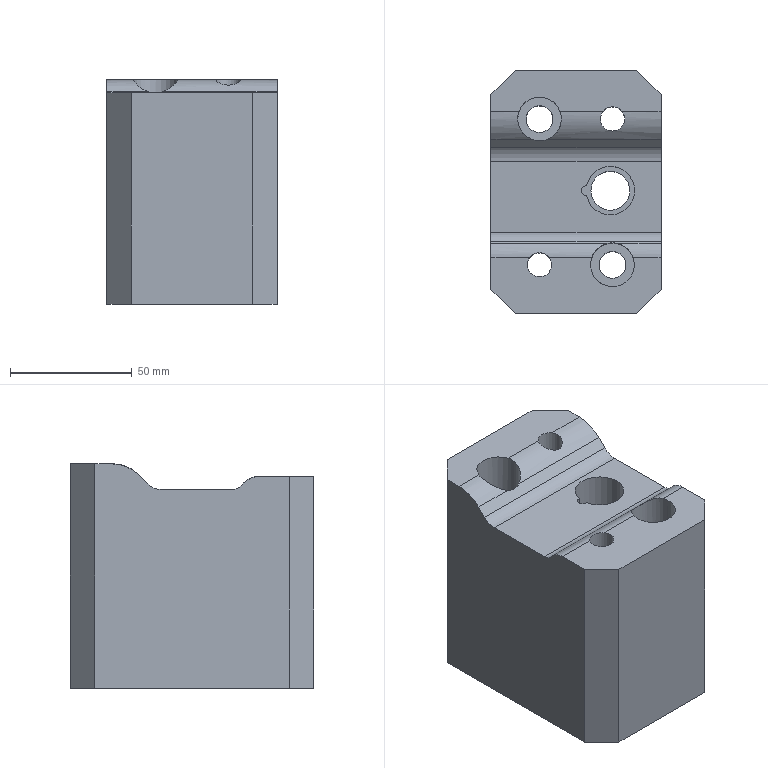Part | NX | features solid 2 | 1 solid | 34 faces | box 70 x 100 x 92.308 mm | volume 508143 mm3 | plane 18 | cylinder 16 | commonest cylinder face diameters 16 x4 10 x3 11 x2 18 x2 32 x2 4 x1
STEP:
#1=CARTESIAN_POINT('',(279.343,-472.51,86.708));
#2=VERTEX_POINT('',#1);
#3=CARTESIAN_POINT('',(279.343,-476.49,86.708));
#4=VERTEX_POINT('',#3);
#5=CARTESIAN_POINT('',(279.143,-474.5,86.708));
#6=DIRECTION('',(0.,0.,1.));
#7=DIRECTION('',(1.,0.,0.));
#8=AXIS2_PLACEMENT_3D('',#5,#6,#7);
#9=CIRCLE('',#8,2.);
#10=EDGE_CURVE('',#2,#4,#9,.T.);
#11=ORIENTED_EDGE('',*,*,#10,.F.);
#12=CARTESIAN_POINT('',(289.143,-474.5,86.708));
#13=DIRECTION('',(0.,0.,1.));
#14=DIRECTION('',(1.,0.,0.));
#15=AXIS2_PLACEMENT_3D('',#12,#13,#14);
#16=CIRCLE('',#15,10.);
#17=EDGE_CURVE('',#2,#4,#16,.F.);
#18=ORIENTED_EDGE('',*,*,#17,.T.);
#19=EDGE_LOOP('',(#11,#18));
#20=FACE_BOUND('',#19,.T.);
#21=CARTESIAN_POINT('',(240.,-491.596,86.708));
#22=VERTEX_POINT('',#21);
#23=CARTESIAN_POINT('',(240.,-462.454,86.708));
#24=VERTEX_POINT('',#23);
#25=CARTESIAN_POINT('',(240.,-475.,86.708));
#26=DIRECTION('',(0.,1.,0.));
#27=VECTOR('',#26,1000.);
#28=LINE('',#25,#27);
#29=EDGE_CURVE('',#22,#24,#28,.T.);
#30=ORIENTED_EDGE('',*,*,#29,.F.);
#31=CARTESIAN_POINT('',(310.,-491.596,86.708));
#32=VERTEX_POINT('',#31);
#33=CARTESIAN_POINT('',(240.,-491.596,86.708));
#34=CARTESIAN_POINT('',(263.333,-491.596,86.708));
#35=CARTESIAN_POINT('',(286.667,-491.596,86.708));
#36=CARTESIAN_POINT('',(310.,-491.596,86.708));
#37=B_SPLINE_CURVE_WITH_KNOTS('',3,(#33,#34,#35,#36),.UNSPECIFIED.,.F.,.F.,(4,4),(0.7902,0.8748),.UNSPECIFIED.);
#38=EDGE_CURVE('',#22,#32,#37,.T.);
#39=ORIENTED_EDGE('',*,*,#38,.T.);
#40=CARTESIAN_POINT('',(310.,-462.454,86.708));
#41=VERTEX_POINT('',#40);
#42=CARTESIAN_POINT('',(310.,-475.,86.708));
#43=DIRECTION('',(0.,-1.,0.));
#44=VECTOR('',#43,1000.);
#45=LINE('',#42,#44);
#46=EDGE_CURVE('',#41,#32,#45,.T.);
#47=ORIENTED_EDGE('',*,*,#46,.F.);
#48=CARTESIAN_POINT('',(310.,-462.454,86.708));
#49=CARTESIAN_POINT('',(286.667,-462.454,86.708));
#50=CARTESIAN_POINT('',(263.333,-462.454,86.708));
#51=CARTESIAN_POINT('',(240.,-462.454,86.708));
#52=B_SPLINE_CURVE_WITH_KNOTS('',3,(#48,#49,#50,#51),.UNSPECIFIED.,.F.,.F.,(4,4),(0.1252,0.2098),.UNSPECIFIED.);
#53=EDGE_CURVE('',#41,#24,#52,.T.);
#54=ORIENTED_EDGE('',*,*,#53,.T.);
#55=EDGE_LOOP('',(#30,#39,#47,#54));
#56=FACE_BOUND('',#55,.T.);
#57=CARTESIAN_POINT('',(426.488,227.578,86.708));
#58=DIRECTION('',(0.,0.,1.));
#59=DIRECTION('',(0.,-1.,0.));
#60=AXIS2_PLACEMENT_3D('',#57,#58,#59);
#61=PLANE('',#60);
#62=ADVANCED_FACE('',(#20,#56),#61,.T.);
#63=CARTESIAN_POINT('',(300.,-525.,5.));
#64=VERTEX_POINT('',#63);
#65=CARTESIAN_POINT('',(300.,-525.,92.008));
#66=VERTEX_POINT('',#65);
#67=CARTESIAN_POINT('',(300.,-525.,10.));
#68=DIRECTION('',(0.,0.,1.));
#69=VECTOR('',#68,1000.);
#70=LINE('',#67,#69);
#71=EDGE_CURVE('',#64,#66,#70,.T.);
#72=ORIENTED_EDGE('',*,*,#71,.T.);
#73=CARTESIAN_POINT('',(250.,-525.,92.008));
#74=VERTEX_POINT('',#73);
#75=CARTESIAN_POINT('',(250.,-525.,92.008));
#76=DIRECTION('',(-1.,0.,0.));
#77=VECTOR('',#76,1000.);
#78=LINE('',#75,#77);
#79=EDGE_CURVE('',#66,#74,#78,.T.);
#80=ORIENTED_EDGE('',*,*,#79,.T.);
#81=CARTESIAN_POINT('',(250.,-525.,5.));
#82=VERTEX_POINT('',#81);
#83=CARTESIAN_POINT('',(250.,-525.,10.));
#84=DIRECTION('',(0.,0.,-1.));
#85=VECTOR('',#84,1000.);
#86=LINE('',#83,#85);
#87=EDGE_CURVE('',#74,#82,#86,.T.);
#88=ORIENTED_EDGE('',*,*,#87,.T.);
#89=CARTESIAN_POINT('',(250.,-525.,5.));
#90=DIRECTION('',(1.,0.,0.));
#91=VECTOR('',#90,1000.);
#92=LINE('',#89,#91);
#93=EDGE_CURVE('',#82,#64,#92,.T.);
#94=ORIENTED_EDGE('',*,*,#93,.T.);
#95=EDGE_LOOP('',(#72,#80,#88,#94));
#96=FACE_BOUND('',#95,.T.);
#97=CARTESIAN_POINT('',(250.,-525.,10.));
#98=DIRECTION('',(0.,-1.,0.));
#99=DIRECTION('',(0.,0.,-1.));
#100=AXIS2_PLACEMENT_3D('',#97,#98,#99);
#101=PLANE('',#100);
#102=ADVANCED_FACE('',(#96),#101,.T.);
#103=CARTESIAN_POINT('',(240.,-515.,5.));
#104=VERTEX_POINT('',#103);
#105=CARTESIAN_POINT('',(240.,-515.,92.008));
#106=VERTEX_POINT('',#105);
#107=CARTESIAN_POINT('',(240.,-515.,10.));
#108=DIRECTION('',(0.,0.,1.));
#109=VECTOR('',#108,1000.);
#110=LINE('',#107,#109);
#111=EDGE_CURVE('',#104,#106,#110,.T.);
#112=ORIENTED_EDGE('',*,*,#111,.T.);
#113=CARTESIAN_POINT('',(240.,-502.176,92.008));
#114=VERTEX_POINT('',#113);
#115=CARTESIAN_POINT('',(240.,-475.,92.008));
#116=DIRECTION('',(0.,1.,0.));
#117=VECTOR('',#116,1000.);
#118=LINE('',#115,#117);
#119=EDGE_CURVE('',#106,#114,#118,.T.);
#120=ORIENTED_EDGE('',*,*,#119,.T.);
#121=CARTESIAN_POINT('',(240.,-496.288,89.423));
#122=VERTEX_POINT('',#121);
#123=CARTESIAN_POINT('',(240.,-502.176,84.008));
#124=DIRECTION('',(-1.,0.,0.));
#125=DIRECTION('',(0.,0.,1.));
#126=AXIS2_PLACEMENT_3D('',#123,#124,#125);
#127=CIRCLE('',#126,8.);
#128=EDGE_CURVE('',#114,#122,#127,.T.);
#129=ORIENTED_EDGE('',*,*,#128,.T.);
#130=CARTESIAN_POINT('',(240.,-495.276,88.323));
#131=VERTEX_POINT('',#130);
#132=CARTESIAN_POINT('',(240.,-446.959,35.79));
#133=DIRECTION('',(0.,0.677,-0.736));
#134=VECTOR('',#133,1000.);
#135=LINE('',#132,#134);
#136=EDGE_CURVE('',#122,#131,#135,.T.);
#137=ORIENTED_EDGE('',*,*,#136,.T.);
#138=CARTESIAN_POINT('',(240.,-491.596,91.708));
#139=DIRECTION('',(-1.,0.,0.));
#140=DIRECTION('',(0.,0.,1.));
#141=AXIS2_PLACEMENT_3D('',#138,#139,#140);
#142=CIRCLE('',#141,5.);
#143=EDGE_CURVE('',#22,#131,#142,.T.);
#144=ORIENTED_EDGE('',*,*,#143,.F.);
#145=ORIENTED_EDGE('',*,*,#29,.T.);
#146=CARTESIAN_POINT('',(240.,-456.76,89.089));
#147=VERTEX_POINT('',#146);
#148=CARTESIAN_POINT('',(240.,-462.454,94.708));
#149=DIRECTION('',(-1.,0.,0.));
#150=DIRECTION('',(0.,0.,1.));
#151=AXIS2_PLACEMENT_3D('',#148,#149,#150);
#152=CIRCLE('',#151,8.);
#153=EDGE_CURVE('',#147,#24,#152,.T.);
#154=ORIENTED_EDGE('',*,*,#153,.F.);
#155=CARTESIAN_POINT('',(240.,-453.348,92.546));
#156=VERTEX_POINT('',#155);
#157=CARTESIAN_POINT('',(240.,-505.299,39.898));
#158=DIRECTION('',(0.,0.7024,0.7118));
#159=VECTOR('',#158,1000.);
#160=LINE('',#157,#159);
#161=EDGE_CURVE('',#147,#156,#160,.T.);
#162=ORIENTED_EDGE('',*,*,#161,.T.);
#163=CARTESIAN_POINT('',(240.,-441.959,97.308));
#164=VERTEX_POINT('',#163);
#165=CARTESIAN_POINT('',(240.,-441.959,81.308));
#166=DIRECTION('',(-1.,0.,0.));
#167=DIRECTION('',(0.,0.,1.));
#168=AXIS2_PLACEMENT_3D('',#165,#166,#167);
#169=CIRCLE('',#168,16.);
#170=EDGE_CURVE('',#156,#164,#169,.T.);
#171=ORIENTED_EDGE('',*,*,#170,.T.);
#172=CARTESIAN_POINT('',(240.,-435.,97.308));
#173=VERTEX_POINT('',#172);
#174=CARTESIAN_POINT('',(240.,-475.,97.308));
#175=DIRECTION('',(0.,1.,0.));
#176=VECTOR('',#175,1000.);
#177=LINE('',#174,#176);
#178=EDGE_CURVE('',#164,#173,#177,.T.);
#179=ORIENTED_EDGE('',*,*,#178,.T.);
#180=CARTESIAN_POINT('',(240.,-435.,5.));
#181=VERTEX_POINT('',#180);
#182=CARTESIAN_POINT('',(240.,-435.,10.));
#183=DIRECTION('',(0.,0.,-1.));
#184=VECTOR('',#183,1000.);
#185=LINE('',#182,#184);
#186=EDGE_CURVE('',#173,#181,#185,.T.);
#187=ORIENTED_EDGE('',*,*,#186,.T.);
#188=CARTESIAN_POINT('',(240.,-475.,5.));
#189=DIRECTION('',(0.,-1.,0.));
#190=VECTOR('',#189,1000.);
#191=LINE('',#188,#190);
#192=EDGE_CURVE('',#181,#104,#191,.T.);
#193=ORIENTED_EDGE('',*,*,#192,.T.);
#194=EDGE_LOOP('',(#112,#120,#129,#137,#144,#145,#154,#162,#171,#179,#187,#193));
#195=FACE_BOUND('',#194,.T.);
#196=CARTESIAN_POINT('',(240.,-475.,10.));
#197=DIRECTION('',(-1.,0.,0.));
#198=DIRECTION('',(0.,0.,1.));
#199=AXIS2_PLACEMENT_3D('',#196,#197,#198);
#200=PLANE('',#199);
#201=ADVANCED_FACE('',(#195),#200,.T.);
#202=CARTESIAN_POINT('',(250.,-425.,5.));
#203=VERTEX_POINT('',#202);
#204=CARTESIAN_POINT('',(250.,-425.,97.308));
#205=VERTEX_POINT('',#204);
#206=CARTESIAN_POINT('',(250.,-425.,10.));
#207=DIRECTION('',(0.,0.,1.));
#208=VECTOR('',#207,1000.);
#209=LINE('',#206,#208);
#210=EDGE_CURVE('',#203,#205,#209,.T.);
#211=ORIENTED_EDGE('',*,*,#210,.T.);
#212=CARTESIAN_POINT('',(300.,-425.,97.308));
#213=VERTEX_POINT('',#212);
#214=CARTESIAN_POINT('',(250.,-425.,97.308));
#215=DIRECTION('',(1.,0.,0.));
#216=VECTOR('',#215,1000.);
#217=LINE('',#214,#216);
#218=EDGE_CURVE('',#205,#213,#217,.T.);
#219=ORIENTED_EDGE('',*,*,#218,.T.);
#220=CARTESIAN_POINT('',(300.,-425.,5.));
#221=VERTEX_POINT('',#220);
#222=CARTESIAN_POINT('',(300.,-425.,10.));
#223=DIRECTION('',(0.,0.,-1.));
#224=VECTOR('',#223,1000.);
#225=LINE('',#222,#224);
#226=EDGE_CURVE('',#213,#221,#225,.T.);
#227=ORIENTED_EDGE('',*,*,#226,.T.);
#228=CARTESIAN_POINT('',(250.,-425.,5.));
#229=DIRECTION('',(-1.,0.,0.));
#230=VECTOR('',#229,1000.);
#231=LINE('',#228,#230);
#232=EDGE_CURVE('',#221,#203,#231,.T.);
#233=ORIENTED_EDGE('',*,*,#232,.T.);
#234=EDGE_LOOP('',(#211,#219,#227,#233));
#235=FACE_BOUND('',#234,.T.);
#236=CARTESIAN_POINT('',(250.,-425.,10.));
#237=DIRECTION('',(0.,1.,0.));
#238=DIRECTION('',(0.,0.,1.));
#239=AXIS2_PLACEMENT_3D('',#236,#237,#238);
#240=PLANE('',#239);
#241=ADVANCED_FACE('',(#235),#240,.T.);
#242=CARTESIAN_POINT('',(310.,-496.288,89.423));
#243=VERTEX_POINT('',#242);
#244=CARTESIAN_POINT('',(310.,-502.176,92.008));
#245=VERTEX_POINT('',#244);
#246=CARTESIAN_POINT('',(310.,-502.176,84.008));
#247=DIRECTION('',(1.,0.,0.));
#248=DIRECTION('',(0.,0.,-1.));
#249=AXIS2_PLACEMENT_3D('',#246,#247,#248);
#250=CIRCLE('',#249,8.);
#251=EDGE_CURVE('',#243,#245,#250,.T.);
#252=ORIENTED_EDGE('',*,*,#251,.T.);
#253=CARTESIAN_POINT('',(310.,-515.,92.008));
#254=VERTEX_POINT('',#253);
#255=CARTESIAN_POINT('',(310.,-475.,92.008));
#256=DIRECTION('',(0.,-1.,0.));
#257=VECTOR('',#256,1000.);
#258=LINE('',#255,#257);
#259=EDGE_CURVE('',#245,#254,#258,.T.);
#260=ORIENTED_EDGE('',*,*,#259,.T.);
#261=CARTESIAN_POINT('',(310.,-515.,5.));
#262=VERTEX_POINT('',#261);
#263=CARTESIAN_POINT('',(310.,-515.,10.));
#264=DIRECTION('',(0.,0.,-1.));
#265=VECTOR('',#264,1000.);
#266=LINE('',#263,#265);
#267=EDGE_CURVE('',#254,#262,#266,.T.);
#268=ORIENTED_EDGE('',*,*,#267,.T.);
#269=CARTESIAN_POINT('',(310.,-435.,5.));
#270=VERTEX_POINT('',#269);
#271=CARTESIAN_POINT('',(310.,-475.,5.));
#272=DIRECTION('',(0.,1.,0.));
#273=VECTOR('',#272,1000.);
#274=LINE('',#271,#273);
#275=EDGE_CURVE('',#262,#270,#274,.T.);
#276=ORIENTED_EDGE('',*,*,#275,.T.);
#277=CARTESIAN_POINT('',(310.,-435.,97.308));
#278=VERTEX_POINT('',#277);
#279=CARTESIAN_POINT('',(310.,-435.,10.));
#280=DIRECTION('',(0.,0.,1.));
#281=VECTOR('',#280,1000.);
#282=LINE('',#279,#281);
#283=EDGE_CURVE('',#270,#278,#282,.T.);
#284=ORIENTED_EDGE('',*,*,#283,.T.);
#285=CARTESIAN_POINT('',(310.,-441.959,97.308));
#286=VERTEX_POINT('',#285);
#287=CARTESIAN_POINT('',(310.,-475.,97.308));
#288=DIRECTION('',(0.,-1.,0.));
#289=VECTOR('',#288,1000.);
#290=LINE('',#287,#289);
#291=EDGE_CURVE('',#278,#286,#290,.T.);
#292=ORIENTED_EDGE('',*,*,#291,.T.);
#293=CARTESIAN_POINT('',(310.,-453.348,92.546));
#294=VERTEX_POINT('',#293);
#295=CARTESIAN_POINT('',(310.,-441.959,81.308));
#296=DIRECTION('',(1.,0.,0.));
#297=DIRECTION('',(0.,0.,-1.));
#298=AXIS2_PLACEMENT_3D('',#295,#296,#297);
#299=CIRCLE('',#298,16.);
#300=EDGE_CURVE('',#286,#294,#299,.T.);
#301=ORIENTED_EDGE('',*,*,#300,.T.);
#302=CARTESIAN_POINT('',(310.,-456.76,89.089));
#303=VERTEX_POINT('',#302);
#304=CARTESIAN_POINT('',(310.,-505.299,39.898));
#305=DIRECTION('',(0.,-0.7024,-0.7118));
#306=VECTOR('',#305,1000.);
#307=LINE('',#304,#306);
#308=EDGE_CURVE('',#294,#303,#307,.T.);
#309=ORIENTED_EDGE('',*,*,#308,.T.);
#310=CARTESIAN_POINT('',(310.,-462.454,94.708));
#311=DIRECTION('',(1.,0.,0.));
#312=DIRECTION('',(0.,0.,-1.));
#313=AXIS2_PLACEMENT_3D('',#310,#311,#312);
#314=CIRCLE('',#313,8.);
#315=EDGE_CURVE('',#41,#303,#314,.T.);
#316=ORIENTED_EDGE('',*,*,#315,.F.);
#317=ORIENTED_EDGE('',*,*,#46,.T.);
#318=CARTESIAN_POINT('',(310.,-495.276,88.323));
#319=VERTEX_POINT('',#318);
#320=CARTESIAN_POINT('',(310.,-491.596,91.708));
#321=DIRECTION('',(1.,0.,0.));
#322=DIRECTION('',(0.,0.,-1.));
#323=AXIS2_PLACEMENT_3D('',#320,#321,#322);
#324=CIRCLE('',#323,5.);
#325=EDGE_CURVE('',#319,#32,#324,.T.);
#326=ORIENTED_EDGE('',*,*,#325,.F.);
#327=CARTESIAN_POINT('',(310.,-446.959,35.79));
#328=DIRECTION('',(0.,-0.677,0.736));
#329=VECTOR('',#328,1000.);
#330=LINE('',#327,#329);
#331=EDGE_CURVE('',#319,#243,#330,.T.);
#332=ORIENTED_EDGE('',*,*,#331,.T.);
#333=EDGE_LOOP('',(#252,#260,#268,#276,#284,#292,#301,#309,#316,#317,#326,#332));
#334=FACE_BOUND('',#333,.T.);
#335=CARTESIAN_POINT('',(310.,-475.,10.));
#336=DIRECTION('',(1.,0.,0.));
#337=DIRECTION('',(0.,0.,-1.));
#338=AXIS2_PLACEMENT_3D('',#335,#336,#337);
#339=PLANE('',#338);
#340=ADVANCED_FACE('',(#334),#339,.T.);
#341=ORIENTED_EDGE('',*,*,#186,.F.);
#342=CARTESIAN_POINT('',(250.,-425.,97.308));
#343=DIRECTION('',(-0.7071,-0.7071,0.));
#344=VECTOR('',#343,1000.);
#345=LINE('',#342,#344);
#346=EDGE_CURVE('',#173,#205,#345,.F.);
#347=ORIENTED_EDGE('',*,*,#346,.T.);
#348=ORIENTED_EDGE('',*,*,#210,.F.);
#349=CARTESIAN_POINT('',(225.,-450.,5.));
#350=DIRECTION('',(-0.7071,-0.7071,0.));
#351=VECTOR('',#350,1000.);
#352=LINE('',#349,#351);
#353=EDGE_CURVE('',#181,#203,#352,.F.);
#354=ORIENTED_EDGE('',*,*,#353,.F.);
#355=EDGE_LOOP('',(#341,#347,#348,#354));
#356=FACE_BOUND('',#355,.T.);
#357=CARTESIAN_POINT('',(250.,-425.,10.));
#358=DIRECTION('',(0.7071,-0.7071,0.));
#359=DIRECTION('',(0.7071,0.7071,0.));
#360=AXIS2_PLACEMENT_3D('',#357,#358,#359);
#361=PLANE('',#360);
#362=ADVANCED_FACE('',(#356),#361,.F.);
#363=ORIENTED_EDGE('',*,*,#226,.F.);
#364=CARTESIAN_POINT('',(310.,-435.,97.308));
#365=DIRECTION('',(-0.7071,0.7071,0.));
#366=VECTOR('',#365,1000.);
#367=LINE('',#364,#366);
#368=EDGE_CURVE('',#213,#278,#367,.F.);
#369=ORIENTED_EDGE('',*,*,#368,.T.);
#370=ORIENTED_EDGE('',*,*,#283,.F.);
#371=CARTESIAN_POINT('',(300.,-425.,5.));
#372=DIRECTION('',(-0.7071,0.7071,0.));
#373=VECTOR('',#372,1000.);
#374=LINE('',#371,#373);
#375=EDGE_CURVE('',#221,#270,#374,.F.);
#376=ORIENTED_EDGE('',*,*,#375,.F.);
#377=EDGE_LOOP('',(#363,#369,#370,#376));
#378=FACE_BOUND('',#377,.T.);
#379=CARTESIAN_POINT('',(310.,-435.,10.));
#380=DIRECTION('',(-0.7071,-0.7071,0.));
#381=DIRECTION('',(0.7071,-0.7071,0.));
#382=AXIS2_PLACEMENT_3D('',#379,#380,#381);
#383=PLANE('',#382);
#384=ADVANCED_FACE('',(#378),#383,.F.);
#385=ORIENTED_EDGE('',*,*,#267,.F.);
#386=CARTESIAN_POINT('',(300.,-525.,92.008));
#387=DIRECTION('',(0.7071,0.7071,0.));
#388=VECTOR('',#387,1000.);
#389=LINE('',#386,#388);
#390=EDGE_CURVE('',#254,#66,#389,.F.);
#391=ORIENTED_EDGE('',*,*,#390,.T.);
#392=ORIENTED_EDGE('',*,*,#71,.F.);
#393=CARTESIAN_POINT('',(300.,-525.,5.));
#394=DIRECTION('',(0.7071,0.7071,0.));
#395=VECTOR('',#394,1000.);
#396=LINE('',#393,#395);
#397=EDGE_CURVE('',#262,#64,#396,.F.);
#398=ORIENTED_EDGE('',*,*,#397,.F.);
#399=EDGE_LOOP('',(#385,#391,#392,#398));
#400=FACE_BOUND('',#399,.T.);
#401=CARTESIAN_POINT('',(300.,-525.,10.));
#402=DIRECTION('',(-0.7071,0.7071,0.));
#403=DIRECTION('',(-0.7071,-0.7071,0.));
#404=AXIS2_PLACEMENT_3D('',#401,#402,#403);
#405=PLANE('',#404);
#406=ADVANCED_FACE('',(#400),#405,.F.);
#407=ORIENTED_EDGE('',*,*,#87,.F.);
#408=CARTESIAN_POINT('',(240.,-515.,92.008));
#409=DIRECTION('',(0.7071,-0.7071,0.));
#410=VECTOR('',#409,1000.);
#411=LINE('',#408,#410);
#412=EDGE_CURVE('',#74,#106,#411,.F.);
#413=ORIENTED_EDGE('',*,*,#412,.T.);
#414=ORIENTED_EDGE('',*,*,#111,.F.);
#415=CARTESIAN_POINT('',(225.,-500.,5.));
#416=DIRECTION('',(0.7071,-0.7071,0.));
#417=VECTOR('',#416,1000.);
#418=LINE('',#415,#417);
#419=EDGE_CURVE('',#82,#104,#418,.F.);
#420=ORIENTED_EDGE('',*,*,#419,.F.);
#421=EDGE_LOOP('',(#407,#413,#414,#420));
#422=FACE_BOUND('',#421,.T.);
#423=CARTESIAN_POINT('',(240.,-515.,10.));
#424=DIRECTION('',(0.7071,0.7071,0.));
#425=DIRECTION('',(-0.7071,0.7071,0.));
#426=AXIS2_PLACEMENT_3D('',#423,#424,#425);
#427=PLANE('',#426);
#428=ADVANCED_FACE('',(#422),#427,.F.);
#429=CARTESIAN_POINT('',(251.,-445.,35.));
#430=VERTEX_POINT('',#429);
#431=CARTESIAN_POINT('',(260.,-445.,35.));
#432=DIRECTION('',(0.,0.,-1.));
#433=DIRECTION('',(-1.,0.,0.));
#434=AXIS2_PLACEMENT_3D('',#431,#432,#433);
#435=CIRCLE('',#434,9.);
#436=EDGE_CURVE('',#430,#430,#435,.T.);
#437=ORIENTED_EDGE('',*,*,#436,.T.);
#438=EDGE_LOOP('',(#437));
#439=FACE_BOUND('',#438,.T.);
#440=CARTESIAN_POINT('',(251.529,-441.959,97.308));
#441=VERTEX_POINT('',#440);
#442=CARTESIAN_POINT('',(268.471,-441.959,97.308));
#443=VERTEX_POINT('',#442);
#444=CARTESIAN_POINT('',(260.,-445.,97.308));
#445=DIRECTION('',(0.,0.,1.));
#446=DIRECTION('',(1.,0.,0.));
#447=AXIS2_PLACEMENT_3D('',#444,#445,#446);
#448=CIRCLE('',#447,9.);
#449=EDGE_CURVE('',#441,#443,#448,.F.);
#450=ORIENTED_EDGE('',*,*,#449,.F.);
#451=CARTESIAN_POINT('',(256.637,-453.348,92.546));
#452=VERTEX_POINT('',#451);
#453=CARTESIAN_POINT('',(256.637,-453.348,92.546));
#454=CARTESIAN_POINT('',(255.56,-452.914,92.985));
#455=CARTESIAN_POINT('',(253.714,-451.707,94.101));
#456=CARTESIAN_POINT('',(251.719,-449.039,95.793));
#457=CARTESIAN_POINT('',(250.778,-445.605,97.037));
#458=CARTESIAN_POINT('',(251.109,-443.129,97.308));
#459=CARTESIAN_POINT('',(251.529,-441.959,97.308));
#460=B_SPLINE_CURVE_WITH_KNOTS('',3,(#453,#454,#455,#456,#457,#458,#459),.UNSPECIFIED.,.F.,.F.,(4,1,1,1,4),(0.,0.003663,0.007327,0.01099,0.01465),.UNSPECIFIED.);
#461=EDGE_CURVE('',#452,#441,#460,.T.);
#462=ORIENTED_EDGE('',*,*,#461,.F.);
#463=CARTESIAN_POINT('',(263.363,-453.348,92.546));
#464=VERTEX_POINT('',#463);
#465=CARTESIAN_POINT('',(260.,-445.,101.006));
#466=DIRECTION('',(0.,-0.7118,0.7024));
#467=DIRECTION('',(0.,-0.7024,-0.7118));
#468=AXIS2_PLACEMENT_3D('',#465,#466,#467);
#469=ELLIPSE('',#468,12.814,9.);
#470=EDGE_CURVE('',#464,#452,#469,.F.);
#471=ORIENTED_EDGE('',*,*,#470,.F.);
#472=CARTESIAN_POINT('',(268.471,-441.959,97.308));
#473=CARTESIAN_POINT('',(268.89,-443.127,97.308));
#474=CARTESIAN_POINT('',(269.222,-445.601,97.038));
#475=CARTESIAN_POINT('',(268.284,-449.033,95.796));
#476=CARTESIAN_POINT('',(266.29,-451.705,94.103));
#477=CARTESIAN_POINT('',(264.438,-452.915,92.985));
#478=CARTESIAN_POINT('',(263.363,-453.348,92.546));
#479=B_SPLINE_CURVE_WITH_KNOTS('',3,(#472,#473,#474,#475,#476,#477,#478),.UNSPECIFIED.,.F.,.F.,(4,1,1,1,4),(0.,0.003667,0.007333,0.011,0.01467),.UNSPECIFIED.);
#480=EDGE_CURVE('',#443,#464,#479,.T.);
#481=ORIENTED_EDGE('',*,*,#480,.F.);
#482=EDGE_LOOP('',(#450,#462,#471,#481));
#483=FACE_BOUND('',#482,.T.);
#484=CARTESIAN_POINT('',(260.,-445.,110.));
#485=DIRECTION('',(0.,0.,-1.));
#486=DIRECTION('',(-1.,0.,0.));
#487=AXIS2_PLACEMENT_3D('',#484,#485,#486);
#488=CYLINDRICAL_SURFACE('',#487,9.);
#489=ADVANCED_FACE('',(#439,#483),#488,.F.);
#490=CARTESIAN_POINT('',(281.,-505.,35.));
#491=VERTEX_POINT('',#490);
#492=CARTESIAN_POINT('',(290.,-505.,35.));
#493=DIRECTION('',(0.,0.,-1.));
#494=DIRECTION('',(-1.,0.,0.));
#495=AXIS2_PLACEMENT_3D('',#492,#493,#494);
#496=CIRCLE('',#495,9.);
#497=EDGE_CURVE('',#491,#491,#496,.T.);
#498=ORIENTED_EDGE('',*,*,#497,.T.);
#499=EDGE_LOOP('',(#498));
#500=FACE_BOUND('',#499,.T.);
#501=CARTESIAN_POINT('',(298.546,-502.176,92.008));
#502=VERTEX_POINT('',#501);
#503=CARTESIAN_POINT('',(281.454,-502.176,92.008));
#504=VERTEX_POINT('',#503);
#505=CARTESIAN_POINT('',(290.,-505.,92.008));
#506=DIRECTION('',(0.,0.,1.));
#507=DIRECTION('',(1.,0.,0.));
#508=AXIS2_PLACEMENT_3D('',#505,#506,#507);
#509=CIRCLE('',#508,9.);
#510=EDGE_CURVE('',#502,#504,#509,.F.);
#511=ORIENTED_EDGE('',*,*,#510,.F.);
#512=CARTESIAN_POINT('',(292.259,-496.288,89.423));
#513=VERTEX_POINT('',#512);
#514=CARTESIAN_POINT('',(292.259,-496.288,89.423));
#515=CARTESIAN_POINT('',(293.737,-496.671,89.84));
#516=CARTESIAN_POINT('',(296.282,-498.07,91.165));
#517=CARTESIAN_POINT('',(298.048,-500.671,92.008));
#518=CARTESIAN_POINT('',(298.546,-502.176,92.008));
#519=B_SPLINE_CURVE_WITH_KNOTS('',3,(#514,#515,#516,#517,#518),.UNSPECIFIED.,.F.,.F.,(4,1,4),(0.,0.00467,0.00934),.UNSPECIFIED.);
#520=EDGE_CURVE('',#513,#502,#519,.T.);
#521=ORIENTED_EDGE('',*,*,#520,.F.);
#522=CARTESIAN_POINT('',(287.741,-496.288,89.423));
#523=VERTEX_POINT('',#522);
#524=CARTESIAN_POINT('',(290.,-505.,98.896));
#525=DIRECTION('',(0.,0.736,0.677));
#526=DIRECTION('',(0.,0.677,-0.736));
#527=AXIS2_PLACEMENT_3D('',#524,#525,#526);
#528=ELLIPSE('',#527,13.295,9.);
#529=EDGE_CURVE('',#523,#513,#528,.F.);
#530=ORIENTED_EDGE('',*,*,#529,.F.);
#531=CARTESIAN_POINT('',(281.454,-502.176,92.008));
#532=CARTESIAN_POINT('',(281.951,-500.673,92.008));
#533=CARTESIAN_POINT('',(283.7,-498.084,91.174));
#534=CARTESIAN_POINT('',(286.268,-496.67,89.839));
#535=CARTESIAN_POINT('',(287.741,-496.288,89.423));
#536=B_SPLINE_CURVE_WITH_KNOTS('',3,(#531,#532,#533,#534,#535),.UNSPECIFIED.,.F.,.F.,(4,1,4),(0.,0.004663,0.009327),.UNSPECIFIED.);
#537=EDGE_CURVE('',#504,#523,#536,.T.);
#538=ORIENTED_EDGE('',*,*,#537,.F.);
#539=EDGE_LOOP('',(#511,#521,#530,#538));
#540=FACE_BOUND('',#539,.T.);
#541=CARTESIAN_POINT('',(290.,-505.,110.));
#542=DIRECTION('',(0.,0.,-1.));
#543=DIRECTION('',(-1.,0.,0.));
#544=AXIS2_PLACEMENT_3D('',#541,#542,#543);
#545=CYLINDRICAL_SURFACE('',#544,9.);
#546=ADVANCED_FACE('',(#500,#540),#545,.F.);
#547=CARTESIAN_POINT('',(285.,-445.,5.));
#548=VERTEX_POINT('',#547);
#549=CARTESIAN_POINT('',(290.,-445.,5.));
#550=DIRECTION('',(0.,0.,-1.));
#551=DIRECTION('',(-1.,0.,0.));
#552=AXIS2_PLACEMENT_3D('',#549,#550,#551);
#553=CIRCLE('',#552,5.);
#554=EDGE_CURVE('',#548,#548,#553,.T.);
#555=ORIENTED_EDGE('',*,*,#554,.T.);
#556=EDGE_LOOP('',(#555));
#557=FACE_BOUND('',#556,.T.);
#558=CARTESIAN_POINT('',(286.031,-441.959,97.308));
#559=VERTEX_POINT('',#558);
#560=CARTESIAN_POINT('',(293.969,-441.959,97.308));
#561=VERTEX_POINT('',#560);
#562=CARTESIAN_POINT('',(290.,-445.,97.308));
#563=DIRECTION('',(0.,0.,1.));
#564=DIRECTION('',(1.,0.,0.));
#565=AXIS2_PLACEMENT_3D('',#562,#563,#564);
#566=CIRCLE('',#565,5.);
#567=EDGE_CURVE('',#559,#561,#566,.F.);
#568=ORIENTED_EDGE('',*,*,#567,.F.);
#569=CARTESIAN_POINT('',(293.969,-441.959,97.308));
#570=CARTESIAN_POINT('',(294.552,-442.72,97.308));
#571=CARTESIAN_POINT('',(295.25,-444.556,97.188));
#572=CARTESIAN_POINT('',(294.683,-447.37,96.446));
#573=CARTESIAN_POINT('',(292.822,-449.433,95.486));
#574=CARTESIAN_POINT('',(290.016,-450.281,94.969));
#575=CARTESIAN_POINT('',(287.18,-449.441,95.483));
#576=CARTESIAN_POINT('',(285.318,-447.367,96.446));
#577=CARTESIAN_POINT('',(284.748,-444.574,97.184));
#578=CARTESIAN_POINT('',(285.448,-442.721,97.308));
#579=CARTESIAN_POINT('',(286.031,-441.959,97.308));
#580=B_SPLINE_CURVE_WITH_KNOTS('',3,(#569,#570,#571,#572,#573,#574,#575,#576,#577,#578,#579),.UNSPECIFIED.,.F.,.F.,(4,1,1,1,1,1,1,1,4),(0.,0.002833,0.005666,0.008499,0.01133,0.01417,0.017,0.01983,0.02266),.UNSPECIFIED.);
#581=EDGE_CURVE('',#561,#559,#580,.T.);
#582=ORIENTED_EDGE('',*,*,#581,.F.);
#583=EDGE_LOOP('',(#568,#582));
#584=FACE_BOUND('',#583,.T.);
#585=CARTESIAN_POINT('',(290.,-445.,110.));
#586=DIRECTION('',(0.,0.,-1.));
#587=DIRECTION('',(-1.,0.,0.));
#588=AXIS2_PLACEMENT_3D('',#585,#586,#587);
#589=CYLINDRICAL_SURFACE('',#588,5.);
#590=ADVANCED_FACE('',(#557,#584),#589,.F.);
#591=CARTESIAN_POINT('',(255.,-505.,5.));
#592=VERTEX_POINT('',#591);
#593=CARTESIAN_POINT('',(260.,-505.,5.));
#594=DIRECTION('',(0.,0.,-1.));
#595=DIRECTION('',(-1.,0.,0.));
#596=AXIS2_PLACEMENT_3D('',#593,#594,#595);
#597=CIRCLE('',#596,5.);
#598=EDGE_CURVE('',#592,#592,#597,.T.);
#599=ORIENTED_EDGE('',*,*,#598,.T.);
#600=EDGE_LOOP('',(#599));
#601=FACE_BOUND('',#600,.T.);
#602=CARTESIAN_POINT('',(264.126,-502.176,92.008));
#603=VERTEX_POINT('',#602);
#604=CARTESIAN_POINT('',(255.874,-502.176,92.008));
#605=VERTEX_POINT('',#604);
#606=CARTESIAN_POINT('',(260.,-505.,92.008));
#607=DIRECTION('',(0.,0.,1.));
#608=DIRECTION('',(1.,0.,0.));
#609=AXIS2_PLACEMENT_3D('',#606,#607,#608);
#610=CIRCLE('',#609,5.);
#611=EDGE_CURVE('',#603,#605,#610,.F.);
#612=ORIENTED_EDGE('',*,*,#611,.F.);
#613=CARTESIAN_POINT('',(255.874,-502.176,92.008));
#614=CARTESIAN_POINT('',(256.799,-500.825,92.008));
#615=CARTESIAN_POINT('',(259.992,-499.175,91.404));
#616=CARTESIAN_POINT('',(263.202,-500.825,92.008));
#617=CARTESIAN_POINT('',(264.126,-502.176,92.008));
#618=B_SPLINE_CURVE_WITH_KNOTS('',3,(#613,#614,#615,#616,#617),.UNSPECIFIED.,.F.,.F.,(4,1,4),(0.,0.004838,0.009677),.UNSPECIFIED.);
#619=EDGE_CURVE('',#605,#603,#618,.T.);
#620=ORIENTED_EDGE('',*,*,#619,.F.);
#621=EDGE_LOOP('',(#612,#620));
#622=FACE_BOUND('',#621,.T.);
#623=CARTESIAN_POINT('',(260.,-505.,110.));
#624=DIRECTION('',(0.,0.,-1.));
#625=DIRECTION('',(-1.,0.,0.));
#626=AXIS2_PLACEMENT_3D('',#623,#624,#625);
#627=CYLINDRICAL_SURFACE('',#626,5.);
#628=ADVANCED_FACE('',(#601,#622),#627,.F.);
#629=CARTESIAN_POINT('',(277.643,-474.5,5.));
#630=VERTEX_POINT('',#629);
#631=CARTESIAN_POINT('',(289.143,-474.5,5.));
#632=DIRECTION('',(0.,0.,-1.));
#633=DIRECTION('',(-1.,0.,0.));
#634=AXIS2_PLACEMENT_3D('',#631,#632,#633);
#635=CIRCLE('',#634,11.5);
#636=EDGE_CURVE('',#630,#630,#635,.F.);
#637=ORIENTED_EDGE('',*,*,#636,.T.);
#638=EDGE_LOOP('',(#637));
#639=FACE_BOUND('',#638,.T.);
#640=ORIENTED_EDGE('',*,*,#598,.F.);
#641=EDGE_LOOP('',(#640));
#642=FACE_BOUND('',#641,.T.);
#643=ORIENTED_EDGE('',*,*,#554,.F.);
#644=EDGE_LOOP('',(#643));
#645=FACE_BOUND('',#644,.T.);
#646=CARTESIAN_POINT('',(284.5,-505.,5.));
#647=VERTEX_POINT('',#646);
#648=CARTESIAN_POINT('',(290.,-505.,5.));
#649=DIRECTION('',(0.,0.,-1.));
#650=DIRECTION('',(-1.,0.,0.));
#651=AXIS2_PLACEMENT_3D('',#648,#649,#650);
#652=CIRCLE('',#651,5.5);
#653=EDGE_CURVE('',#647,#647,#652,.T.);
#654=ORIENTED_EDGE('',*,*,#653,.F.);
#655=EDGE_LOOP('',(#654));
#656=FACE_BOUND('',#655,.T.);
#657=CARTESIAN_POINT('',(254.5,-445.,5.));
#658=VERTEX_POINT('',#657);
#659=CARTESIAN_POINT('',(260.,-445.,5.));
#660=DIRECTION('',(0.,0.,-1.));
#661=DIRECTION('',(-1.,0.,0.));
#662=AXIS2_PLACEMENT_3D('',#659,#660,#661);
#663=CIRCLE('',#662,5.5);
#664=EDGE_CURVE('',#658,#658,#663,.T.);
#665=ORIENTED_EDGE('',*,*,#664,.F.);
#666=EDGE_LOOP('',(#665));
#667=FACE_BOUND('',#666,.T.);
#668=ORIENTED_EDGE('',*,*,#192,.F.);
#669=ORIENTED_EDGE('',*,*,#353,.T.);
#670=ORIENTED_EDGE('',*,*,#232,.F.);
#671=ORIENTED_EDGE('',*,*,#375,.T.);
#672=ORIENTED_EDGE('',*,*,#275,.F.);
#673=ORIENTED_EDGE('',*,*,#397,.T.);
#674=ORIENTED_EDGE('',*,*,#93,.F.);
#675=ORIENTED_EDGE('',*,*,#419,.T.);
#676=EDGE_LOOP('',(#668,#669,#670,#671,#672,#673,#674,#675));
#677=FACE_BOUND('',#676,.T.);
#678=CARTESIAN_POINT('',(250.,-475.,5.));
#679=DIRECTION('',(0.,0.,-1.));
#680=DIRECTION('',(-1.,0.,0.));
#681=AXIS2_PLACEMENT_3D('',#678,#679,#680);
#682=PLANE('',#681);
#683=ADVANCED_FACE('',(#639,#642,#645,#656,#667,#677),#682,.T.);
#684=ORIENTED_EDGE('',*,*,#664,.T.);
#685=EDGE_LOOP('',(#684));
#686=FACE_BOUND('',#685,.T.);
#687=CARTESIAN_POINT('',(254.5,-445.,35.));
#688=VERTEX_POINT('',#687);
#689=CARTESIAN_POINT('',(260.,-445.,35.));
#690=DIRECTION('',(0.,0.,-1.));
#691=DIRECTION('',(-1.,0.,0.));
#692=AXIS2_PLACEMENT_3D('',#689,#690,#691);
#693=CIRCLE('',#692,5.5);
#694=EDGE_CURVE('',#688,#688,#693,.T.);
#695=ORIENTED_EDGE('',*,*,#694,.F.);
#696=EDGE_LOOP('',(#695));
#697=FACE_BOUND('',#696,.T.);
#698=CARTESIAN_POINT('',(260.,-445.,5.));
#699=DIRECTION('',(0.,0.,-1.));
#700=DIRECTION('',(-1.,0.,0.));
#701=AXIS2_PLACEMENT_3D('',#698,#699,#700);
#702=CYLINDRICAL_SURFACE('',#701,5.5);
#703=ADVANCED_FACE('',(#686,#697),#702,.F.);
#704=ORIENTED_EDGE('',*,*,#694,.T.);
#705=EDGE_LOOP('',(#704));
#706=FACE_BOUND('',#705,.T.);
#707=ORIENTED_EDGE('',*,*,#436,.F.);
#708=EDGE_LOOP('',(#707));
#709=FACE_BOUND('',#708,.T.);
#710=CARTESIAN_POINT('',(260.,-445.,35.));
#711=DIRECTION('',(0.,0.,-1.));
#712=DIRECTION('',(-1.,0.,0.));
#713=AXIS2_PLACEMENT_3D('',#710,#711,#712);
#714=PLANE('',#713);
#715=ADVANCED_FACE('',(#706,#709),#714,.F.);
#716=ORIENTED_EDGE('',*,*,#653,.T.);
#717=EDGE_LOOP('',(#716));
#718=FACE_BOUND('',#717,.T.);
#719=CARTESIAN_POINT('',(284.5,-505.,35.));
#720=VERTEX_POINT('',#719);
#721=CARTESIAN_POINT('',(290.,-505.,35.));
#722=DIRECTION('',(0.,0.,-1.));
#723=DIRECTION('',(-1.,0.,0.));
#724=AXIS2_PLACEMENT_3D('',#721,#722,#723);
#725=CIRCLE('',#724,5.5);
#726=EDGE_CURVE('',#720,#720,#725,.T.);
#727=ORIENTED_EDGE('',*,*,#726,.F.);
#728=EDGE_LOOP('',(#727));
#729=FACE_BOUND('',#728,.T.);
#730=CARTESIAN_POINT('',(290.,-505.,5.));
#731=DIRECTION('',(0.,0.,-1.));
#732=DIRECTION('',(-1.,0.,0.));
#733=AXIS2_PLACEMENT_3D('',#730,#731,#732);
#734=CYLINDRICAL_SURFACE('',#733,5.5);
#735=ADVANCED_FACE('',(#718,#729),#734,.F.);
#736=ORIENTED_EDGE('',*,*,#726,.T.);
#737=EDGE_LOOP('',(#736));
#738=FACE_BOUND('',#737,.T.);
#739=ORIENTED_EDGE('',*,*,#497,.F.);
#740=EDGE_LOOP('',(#739));
#741=FACE_BOUND('',#740,.T.);
#742=CARTESIAN_POINT('',(290.,-505.,35.));
#743=DIRECTION('',(0.,0.,-1.));
#744=DIRECTION('',(-1.,0.,0.));
#745=AXIS2_PLACEMENT_3D('',#742,#743,#744);
#746=PLANE('',#745);
#747=ADVANCED_FACE('',(#738,#741),#746,.F.);
#748=ORIENTED_EDGE('',*,*,#161,.F.);
#749=CARTESIAN_POINT('',(240.,-456.76,89.089));
#750=CARTESIAN_POINT('',(263.333,-456.76,89.089));
#751=CARTESIAN_POINT('',(286.667,-456.76,89.089));
#752=CARTESIAN_POINT('',(310.,-456.76,89.089));
#753=B_SPLINE_CURVE_WITH_KNOTS('',3,(#749,#750,#751,#752),.UNSPECIFIED.,.F.,.F.,(4,4),(0.7902,0.8748),.UNSPECIFIED.);
#754=EDGE_CURVE('',#303,#147,#753,.F.);
#755=ORIENTED_EDGE('',*,*,#754,.F.);
#756=ORIENTED_EDGE('',*,*,#308,.F.);
#757=CARTESIAN_POINT('',(310.,-453.348,92.546));
#758=CARTESIAN_POINT('',(294.454,-453.348,92.546));
#759=CARTESIAN_POINT('',(278.908,-453.348,92.546));
#760=CARTESIAN_POINT('',(263.363,-453.348,92.546));
#761=B_SPLINE_CURVE_WITH_KNOTS('',3,(#757,#758,#759,#760),.UNSPECIFIED.,.F.,.F.,(4,4),(0.1252,0.1816),.UNSPECIFIED.);
#762=EDGE_CURVE('',#294,#464,#761,.T.);
#763=ORIENTED_EDGE('',*,*,#762,.T.);
#764=ORIENTED_EDGE('',*,*,#470,.T.);
#765=CARTESIAN_POINT('',(256.637,-453.348,92.546));
#766=CARTESIAN_POINT('',(251.092,-453.348,92.546));
#767=CARTESIAN_POINT('',(245.546,-453.348,92.546));
#768=CARTESIAN_POINT('',(240.,-453.348,92.546));
#769=B_SPLINE_CURVE_WITH_KNOTS('',3,(#765,#766,#767,#768),.UNSPECIFIED.,.F.,.F.,(4,4),(0.1897,0.2098),.UNSPECIFIED.);
#770=EDGE_CURVE('',#452,#156,#769,.T.);
#771=ORIENTED_EDGE('',*,*,#770,.T.);
#772=EDGE_LOOP('',(#748,#755,#756,#763,#764,#771));
#773=FACE_BOUND('',#772,.T.);
#774=CARTESIAN_POINT('',(513.762,-526.912,17.996));
#775=DIRECTION('',(0.,-0.7118,0.7024));
#776=DIRECTION('',(0.,-0.7024,-0.7118));
#777=AXIS2_PLACEMENT_3D('',#774,#775,#776);
#778=PLANE('',#777);
#779=ADVANCED_FACE('',(#773),#778,.T.);
#780=ORIENTED_EDGE('',*,*,#136,.F.);
#781=CARTESIAN_POINT('',(240.,-496.288,89.423));
#782=CARTESIAN_POINT('',(255.914,-496.288,89.423));
#783=CARTESIAN_POINT('',(271.828,-496.288,89.423));
#784=CARTESIAN_POINT('',(287.741,-496.288,89.423));
#785=B_SPLINE_CURVE_WITH_KNOTS('',3,(#781,#782,#783,#784),.UNSPECIFIED.,.F.,.F.,(4,4),(0.7902,0.8479),.UNSPECIFIED.);
#786=EDGE_CURVE('',#122,#523,#785,.T.);
#787=ORIENTED_EDGE('',*,*,#786,.T.);
#788=ORIENTED_EDGE('',*,*,#529,.T.);
#789=CARTESIAN_POINT('',(292.259,-496.288,89.423));
#790=CARTESIAN_POINT('',(298.172,-496.288,89.423));
#791=CARTESIAN_POINT('',(304.086,-496.288,89.423));
#792=CARTESIAN_POINT('',(310.,-496.288,89.423));
#793=B_SPLINE_CURVE_WITH_KNOTS('',3,(#789,#790,#791,#792),.UNSPECIFIED.,.F.,.F.,(4,4),(0.8533,0.8748),.UNSPECIFIED.);
#794=EDGE_CURVE('',#513,#243,#793,.T.);
#795=ORIENTED_EDGE('',*,*,#794,.T.);
#796=ORIENTED_EDGE('',*,*,#331,.F.);
#797=CARTESIAN_POINT('',(310.,-495.276,88.323));
#798=CARTESIAN_POINT('',(286.667,-495.276,88.323));
#799=CARTESIAN_POINT('',(263.333,-495.276,88.323));
#800=CARTESIAN_POINT('',(240.,-495.276,88.323));
#801=B_SPLINE_CURVE_WITH_KNOTS('',3,(#797,#798,#799,#800),.UNSPECIFIED.,.F.,.F.,(4,4),(0.1252,0.2098),.UNSPECIFIED.);
#802=EDGE_CURVE('',#319,#131,#801,.T.);
#803=ORIENTED_EDGE('',*,*,#802,.T.);
#804=EDGE_LOOP('',(#780,#787,#788,#795,#796,#803));
#805=FACE_BOUND('',#804,.T.);
#806=CARTESIAN_POINT('',(-513.463,-424.358,11.217));
#807=DIRECTION('',(0.,0.736,0.677));
#808=DIRECTION('',(0.,-0.677,0.736));
#809=AXIS2_PLACEMENT_3D('',#806,#807,#808);
#810=PLANE('',#809);
#811=ADVANCED_FACE('',(#805),#810,.T.);
#812=ORIENTED_EDGE('',*,*,#178,.F.);
#813=CARTESIAN_POINT('',(240.,-441.959,97.308));
#814=CARTESIAN_POINT('',(243.843,-441.959,97.308));
#815=CARTESIAN_POINT('',(247.686,-441.959,97.308));
#816=CARTESIAN_POINT('',(251.529,-441.959,97.308));
#817=B_SPLINE_CURVE_WITH_KNOTS('',3,(#813,#814,#815,#816),.UNSPECIFIED.,.F.,.F.,(4,4),(0.7902,0.8041),.UNSPECIFIED.);
#818=EDGE_CURVE('',#164,#441,#817,.T.);
#819=ORIENTED_EDGE('',*,*,#818,.T.);
#820=ORIENTED_EDGE('',*,*,#449,.T.);
#821=CARTESIAN_POINT('',(268.471,-441.959,97.308));
#822=CARTESIAN_POINT('',(274.324,-441.959,97.308));
#823=CARTESIAN_POINT('',(280.177,-441.959,97.308));
#824=CARTESIAN_POINT('',(286.031,-441.959,97.308));
#825=B_SPLINE_CURVE_WITH_KNOTS('',3,(#821,#822,#823,#824),.UNSPECIFIED.,.F.,.F.,(4,4),(0.8246,0.8458),.UNSPECIFIED.);
#826=EDGE_CURVE('',#443,#559,#825,.T.);
#827=ORIENTED_EDGE('',*,*,#826,.T.);
#828=ORIENTED_EDGE('',*,*,#567,.T.);
#829=CARTESIAN_POINT('',(293.969,-441.959,97.308));
#830=CARTESIAN_POINT('',(299.313,-441.959,97.308));
#831=CARTESIAN_POINT('',(304.656,-441.959,97.308));
#832=CARTESIAN_POINT('',(310.,-441.959,97.308));
#833=B_SPLINE_CURVE_WITH_KNOTS('',3,(#829,#830,#831,#832),.UNSPECIFIED.,.F.,.F.,(4,4),(0.8554,0.8748),.UNSPECIFIED.);
#834=EDGE_CURVE('',#561,#286,#833,.T.);
#835=ORIENTED_EDGE('',*,*,#834,.T.);
#836=ORIENTED_EDGE('',*,*,#291,.F.);
#837=ORIENTED_EDGE('',*,*,#368,.F.);
#838=ORIENTED_EDGE('',*,*,#218,.F.);
#839=ORIENTED_EDGE('',*,*,#346,.F.);
#840=EDGE_LOOP('',(#812,#819,#820,#827,#828,#835,#836,#837,#838,#839));
#841=FACE_BOUND('',#840,.T.);
#842=CARTESIAN_POINT('',(532.124,-754.014,97.308));
#843=DIRECTION('',(0.,0.,1.));
#844=DIRECTION('',(0.,-1.,0.));
#845=AXIS2_PLACEMENT_3D('',#842,#843,#844);
#846=PLANE('',#845);
#847=ADVANCED_FACE('',(#841),#846,.T.);
#848=ORIENTED_EDGE('',*,*,#170,.F.);
#849=ORIENTED_EDGE('',*,*,#770,.F.);
#850=ORIENTED_EDGE('',*,*,#461,.T.);
#851=ORIENTED_EDGE('',*,*,#818,.F.);
#852=EDGE_LOOP('',(#848,#849,#850,#851));
#853=FACE_BOUND('',#852,.T.);
#854=CARTESIAN_POINT('',(-6000414.,-441.959,81.308));
#855=DIRECTION('',(1.,0.,0.));
#856=DIRECTION('',(0.,0.,1.));
#857=AXIS2_PLACEMENT_3D('',#854,#855,#856);
#858=CYLINDRICAL_SURFACE('',#857,16.);
#859=ADVANCED_FACE('',(#853),#858,.T.);
#860=ORIENTED_EDGE('',*,*,#300,.F.);
#861=ORIENTED_EDGE('',*,*,#834,.F.);
#862=ORIENTED_EDGE('',*,*,#581,.T.);
#863=ORIENTED_EDGE('',*,*,#826,.F.);
#864=ORIENTED_EDGE('',*,*,#480,.T.);
#865=ORIENTED_EDGE('',*,*,#762,.F.);
#866=EDGE_LOOP('',(#860,#861,#862,#863,#864,#865));
#867=FACE_BOUND('',#866,.T.);
#868=CARTESIAN_POINT('',(-6000414.,-441.959,81.308));
#869=DIRECTION('',(1.,0.,0.));
#870=DIRECTION('',(0.,0.,1.));
#871=AXIS2_PLACEMENT_3D('',#868,#869,#870);
#872=CYLINDRICAL_SURFACE('',#871,16.);
#873=ADVANCED_FACE('',(#867),#872,.T.);
#874=ORIENTED_EDGE('',*,*,#259,.F.);
#875=CARTESIAN_POINT('',(310.,-502.176,92.008));
#876=CARTESIAN_POINT('',(306.182,-502.176,92.008));
#877=CARTESIAN_POINT('',(302.364,-502.176,92.008));
#878=CARTESIAN_POINT('',(298.546,-502.176,92.008));
#879=B_SPLINE_CURVE_WITH_KNOTS('',3,(#875,#876,#877,#878),.UNSPECIFIED.,.F.,.F.,(4,4),(0.1252,0.1391),.UNSPECIFIED.);
#880=EDGE_CURVE('',#245,#502,#879,.T.);
#881=ORIENTED_EDGE('',*,*,#880,.T.);
#882=ORIENTED_EDGE('',*,*,#510,.T.);
#883=CARTESIAN_POINT('',(281.454,-502.176,92.008));
#884=CARTESIAN_POINT('',(275.678,-502.176,92.008));
#885=CARTESIAN_POINT('',(269.902,-502.176,92.008));
#886=CARTESIAN_POINT('',(264.126,-502.176,92.008));
#887=B_SPLINE_CURVE_WITH_KNOTS('',3,(#883,#884,#885,#886),.UNSPECIFIED.,.F.,.F.,(4,4),(0.1597,0.1806),.UNSPECIFIED.);
#888=EDGE_CURVE('',#504,#603,#887,.T.);
#889=ORIENTED_EDGE('',*,*,#888,.T.);
#890=ORIENTED_EDGE('',*,*,#611,.T.);
#891=CARTESIAN_POINT('',(255.874,-502.176,92.008));
#892=CARTESIAN_POINT('',(250.582,-502.176,92.008));
#893=CARTESIAN_POINT('',(245.291,-502.176,92.008));
#894=CARTESIAN_POINT('',(240.,-502.176,92.008));
#895=B_SPLINE_CURVE_WITH_KNOTS('',3,(#891,#892,#893,#894),.UNSPECIFIED.,.F.,.F.,(4,4),(0.1906,0.2098),.UNSPECIFIED.);
#896=EDGE_CURVE('',#605,#114,#895,.T.);
#897=ORIENTED_EDGE('',*,*,#896,.T.);
#898=ORIENTED_EDGE('',*,*,#119,.F.);
#899=ORIENTED_EDGE('',*,*,#412,.F.);
#900=ORIENTED_EDGE('',*,*,#79,.F.);
#901=ORIENTED_EDGE('',*,*,#390,.F.);
#902=EDGE_LOOP('',(#874,#881,#882,#889,#890,#897,#898,#899,#900,#901));
#903=FACE_BOUND('',#902,.T.);
#904=CARTESIAN_POINT('',(575.068,183.357,92.008));
#905=DIRECTION('',(0.,0.,1.));
#906=DIRECTION('',(0.,-1.,0.));
#907=AXIS2_PLACEMENT_3D('',#904,#905,#906);
#908=PLANE('',#907);
#909=ADVANCED_FACE('',(#903),#908,.T.);
#910=ORIENTED_EDGE('',*,*,#251,.F.);
#911=ORIENTED_EDGE('',*,*,#794,.F.);
#912=ORIENTED_EDGE('',*,*,#520,.T.);
#913=ORIENTED_EDGE('',*,*,#880,.F.);
#914=EDGE_LOOP('',(#910,#911,#912,#913));
#915=FACE_BOUND('',#914,.T.);
#916=CARTESIAN_POINT('',(6000413.634,-502.176,84.008));
#917=DIRECTION('',(-1.,0.,0.));
#918=DIRECTION('',(0.,0.,-1.));
#919=AXIS2_PLACEMENT_3D('',#916,#917,#918);
#920=CYLINDRICAL_SURFACE('',#919,8.);
#921=ADVANCED_FACE('',(#915),#920,.T.);
#922=ORIENTED_EDGE('',*,*,#128,.F.);
#923=ORIENTED_EDGE('',*,*,#896,.F.);
#924=ORIENTED_EDGE('',*,*,#619,.T.);
#925=ORIENTED_EDGE('',*,*,#888,.F.);
#926=ORIENTED_EDGE('',*,*,#537,.T.);
#927=ORIENTED_EDGE('',*,*,#786,.F.);
#928=EDGE_LOOP('',(#922,#923,#924,#925,#926,#927));
#929=FACE_BOUND('',#928,.T.);
#930=CARTESIAN_POINT('',(6000413.634,-502.176,84.008));
#931=DIRECTION('',(-1.,0.,0.));
#932=DIRECTION('',(0.,0.,-1.));
#933=AXIS2_PLACEMENT_3D('',#930,#931,#932);
#934=CYLINDRICAL_SURFACE('',#933,8.);
#935=ADVANCED_FACE('',(#929),#934,.T.);
#936=ORIENTED_EDGE('',*,*,#754,.T.);
#937=ORIENTED_EDGE('',*,*,#153,.T.);
#938=ORIENTED_EDGE('',*,*,#53,.F.);
#939=ORIENTED_EDGE('',*,*,#315,.T.);
#940=EDGE_LOOP('',(#936,#937,#938,#939));
#941=FACE_BOUND('',#940,.T.);
#942=CARTESIAN_POINT('',(-6000414.,-462.454,94.708));
#943=DIRECTION('',(1.,0.,0.));
#944=DIRECTION('',(0.,0.,1.));
#945=AXIS2_PLACEMENT_3D('',#942,#943,#944);
#946=CYLINDRICAL_SURFACE('',#945,8.);
#947=ADVANCED_FACE('',(#941),#946,.F.);
#948=ORIENTED_EDGE('',*,*,#38,.F.);
#949=ORIENTED_EDGE('',*,*,#143,.T.);
#950=ORIENTED_EDGE('',*,*,#802,.F.);
#951=ORIENTED_EDGE('',*,*,#325,.T.);
#952=EDGE_LOOP('',(#948,#949,#950,#951));
#953=FACE_BOUND('',#952,.T.);
#954=CARTESIAN_POINT('',(6000413.634,-491.596,91.708));
#955=DIRECTION('',(-1.,0.,0.));
#956=DIRECTION('',(0.,0.,-1.));
#957=AXIS2_PLACEMENT_3D('',#954,#955,#956);
#958=CYLINDRICAL_SURFACE('',#957,5.);
#959=ADVANCED_FACE('',(#953),#958,.F.);
#960=ORIENTED_EDGE('',*,*,#636,.F.);
#961=EDGE_LOOP('',(#960));
#962=FACE_BOUND('',#961,.T.);
#963=CARTESIAN_POINT('',(300.643,-474.5,47.));
#964=VERTEX_POINT('',#963);
#965=CARTESIAN_POINT('',(289.143,-474.5,47.));
#966=DIRECTION('',(0.,0.,1.));
#967=DIRECTION('',(1.,0.,0.));
#968=AXIS2_PLACEMENT_3D('',#965,#966,#967);
#969=CIRCLE('',#968,11.5);
#970=EDGE_CURVE('',#964,#964,#969,.T.);
#971=ORIENTED_EDGE('',*,*,#970,.T.);
#972=EDGE_LOOP('',(#971));
#973=FACE_BOUND('',#972,.T.);
#974=CARTESIAN_POINT('',(289.143,-474.5,-13.));
#975=DIRECTION('',(0.,0.,1.));
#976=DIRECTION('',(1.,0.,0.));
#977=AXIS2_PLACEMENT_3D('',#974,#975,#976);
#978=CYLINDRICAL_SURFACE('',#977,11.5);
#979=ADVANCED_FACE('',(#962,#973),#978,.F.);
#980=CARTESIAN_POINT('',(297.143,-474.5,47.));
#981=VERTEX_POINT('',#980);
#982=CARTESIAN_POINT('',(289.143,-474.5,47.));
#983=DIRECTION('',(0.,0.,1.));
#984=DIRECTION('',(1.,0.,0.));
#985=AXIS2_PLACEMENT_3D('',#982,#983,#984);
#986=CIRCLE('',#985,8.);
#987=EDGE_CURVE('',#981,#981,#986,.T.);
#988=ORIENTED_EDGE('',*,*,#987,.T.);
#989=EDGE_LOOP('',(#988));
#990=FACE_BOUND('',#989,.T.);
#991=ORIENTED_EDGE('',*,*,#970,.F.);
#992=EDGE_LOOP('',(#991));
#993=FACE_BOUND('',#992,.T.);
#994=CARTESIAN_POINT('',(289.143,-474.5,47.));
#995=DIRECTION('',(0.,0.,1.));
#996=DIRECTION('',(1.,0.,0.));
#997=AXIS2_PLACEMENT_3D('',#994,#995,#996);
#998=PLANE('',#997);
#999=ADVANCED_FACE('',(#990,#993),#998,.F.);
#1000=CARTESIAN_POINT('',(297.143,-474.5,67.));
#1001=VERTEX_POINT('',#1000);
#1002=CARTESIAN_POINT('',(289.143,-474.5,67.));
#1003=DIRECTION('',(0.,0.,1.));
#1004=DIRECTION('',(1.,0.,0.));
#1005=AXIS2_PLACEMENT_3D('',#1002,#1003,#1004);
#1006=CIRCLE('',#1005,8.);
#1007=EDGE_CURVE('',#1001,#1001,#1006,.T.);
#1008=ORIENTED_EDGE('',*,*,#1007,.T.);
#1009=EDGE_LOOP('',(#1008));
#1010=FACE_BOUND('',#1009,.T.);
#1011=ORIENTED_EDGE('',*,*,#987,.F.);
#1012=EDGE_LOOP('',(#1011));
#1013=FACE_BOUND('',#1012,.T.);
#1014=CARTESIAN_POINT('',(289.143,-474.5,17.));
#1015=DIRECTION('',(0.,0.,1.));
#1016=DIRECTION('',(1.,0.,0.));
#1017=AXIS2_PLACEMENT_3D('',#1014,#1015,#1016);
#1018=CYLINDRICAL_SURFACE('',#1017,8.);
#1019=ADVANCED_FACE('',(#1010,#1013),#1018,.F.);
#1020=CARTESIAN_POINT('',(279.343,-472.51,67.));
#1021=VERTEX_POINT('',#1020);
#1022=CARTESIAN_POINT('',(279.343,-472.51,267.));
#1023=DIRECTION('',(0.,0.,-1.));
#1024=VECTOR('',#1023,1000.);
#1025=LINE('',#1022,#1024);
#1026=EDGE_CURVE('',#1021,#2,#1025,.F.);
#1027=ORIENTED_EDGE('',*,*,#1026,.F.);
#1028=CARTESIAN_POINT('',(279.343,-476.49,67.));
#1029=VERTEX_POINT('',#1028);
#1030=CARTESIAN_POINT('',(289.143,-474.5,67.));
#1031=DIRECTION('',(0.,0.,1.));
#1032=DIRECTION('',(-1.,0.,0.));
#1033=AXIS2_PLACEMENT_3D('',#1030,#1031,#1032);
#1034=CIRCLE('',#1033,10.);
#1035=EDGE_CURVE('',#1029,#1021,#1034,.T.);
#1036=ORIENTED_EDGE('',*,*,#1035,.F.);
#1037=CARTESIAN_POINT('',(279.343,-476.49,267.));
#1038=DIRECTION('',(0.,0.,-1.));
#1039=VECTOR('',#1038,1000.);
#1040=LINE('',#1037,#1039);
#1041=EDGE_CURVE('',#4,#1029,#1040,.T.);
#1042=ORIENTED_EDGE('',*,*,#1041,.F.);
#1043=ORIENTED_EDGE('',*,*,#17,.F.);
#1044=EDGE_LOOP('',(#1027,#1036,#1042,#1043));
#1045=FACE_BOUND('',#1044,.T.);
#1046=CARTESIAN_POINT('',(289.143,-474.5,267.));
#1047=DIRECTION('',(0.,0.,-1.));
#1048=DIRECTION('',(-1.,0.,0.));
#1049=AXIS2_PLACEMENT_3D('',#1046,#1047,#1048);
#1050=CYLINDRICAL_SURFACE('',#1049,10.);
#1051=ADVANCED_FACE('',(#1045),#1050,.F.);
#1052=ORIENTED_EDGE('',*,*,#1035,.T.);
#1053=CARTESIAN_POINT('',(279.143,-474.5,67.));
#1054=DIRECTION('',(0.,0.,1.));
#1055=DIRECTION('',(1.,0.,0.));
#1056=AXIS2_PLACEMENT_3D('',#1053,#1054,#1055);
#1057=CIRCLE('',#1056,2.);
#1058=EDGE_CURVE('',#1021,#1029,#1057,.T.);
#1059=ORIENTED_EDGE('',*,*,#1058,.T.);
#1060=EDGE_LOOP('',(#1052,#1059));
#1061=FACE_BOUND('',#1060,.T.);
#1062=ORIENTED_EDGE('',*,*,#1007,.F.);
#1063=EDGE_LOOP('',(#1062));
#1064=FACE_BOUND('',#1063,.T.);
#1065=CARTESIAN_POINT('',(284.143,-474.5,67.));
#1066=DIRECTION('',(0.,0.,1.));
#1067=DIRECTION('',(1.,0.,0.));
#1068=AXIS2_PLACEMENT_3D('',#1065,#1066,#1067);
#1069=PLANE('',#1068);
#1070=ADVANCED_FACE('',(#1061,#1064),#1069,.T.);
#1071=ORIENTED_EDGE('',*,*,#1026,.T.);
#1072=ORIENTED_EDGE('',*,*,#10,.T.);
#1073=ORIENTED_EDGE('',*,*,#1041,.T.);
#1074=ORIENTED_EDGE('',*,*,#1058,.F.);
#1075=EDGE_LOOP('',(#1071,#1072,#1073,#1074));
#1076=FACE_BOUND('',#1075,.T.);
#1077=CARTESIAN_POINT('',(279.143,-474.5,67.));
#1078=DIRECTION('',(0.,0.,1.));
#1079=DIRECTION('',(1.,0.,0.));
#1080=AXIS2_PLACEMENT_3D('',#1077,#1078,#1079);
#1081=CYLINDRICAL_SURFACE('',#1080,2.);
#1082=ADVANCED_FACE('',(#1076),#1081,.F.);
#1083=CLOSED_SHELL('',(#62,#102,#201,#241,#340,#362,#384,#406,#428,#489,#546,#590,#628,#683,#703,#715,#735,#747,#779,#811,#847,#859,#873,#909,#921,#935,#947,#959,#979,#999,#1019,#1051,#1070,#1082));
#1084=MANIFOLD_SOLID_BREP('',#1083);
#1085=(LENGTH_UNIT()NAMED_UNIT(*)SI_UNIT(.MILLI.,.METRE.));
#1086=UNCERTAINTY_MEASURE_WITH_UNIT(LENGTH_MEASURE(0.0508),#1085,'','');
#1087=(NAMED_UNIT(*)PLANE_ANGLE_UNIT()SI_UNIT($,.RADIAN.));
#1088=(NAMED_UNIT(*)SI_UNIT($,.STERADIAN.)SOLID_ANGLE_UNIT());
#1089=(GEOMETRIC_REPRESENTATION_CONTEXT(3)GLOBAL_UNCERTAINTY_ASSIGNED_CONTEXT((#1086))GLOBAL_UNIT_ASSIGNED_CONTEXT((#1085,#1087,#1088))REPRESENTATION_CONTEXT('',''));
#1090=ADVANCED_BREP_SHAPE_REPRESENTATION('',(#1084),#1089);